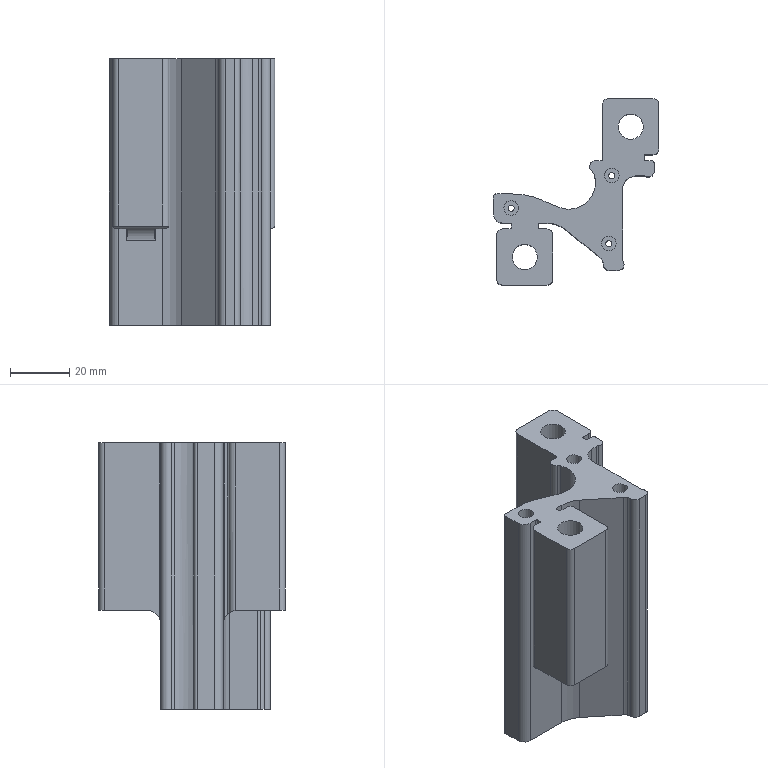Part | NX | features PU-4 2 | 1 solid | 77 faces | box 56.031 x 63.075 x 90 mm | volume 95636 mm3 | plane 32 | cylinder 30 | spline 15 | commonest cylinder face diameters 4 x8 1 x7 2.101 x3 5 x3 2 x2 8.506 x2